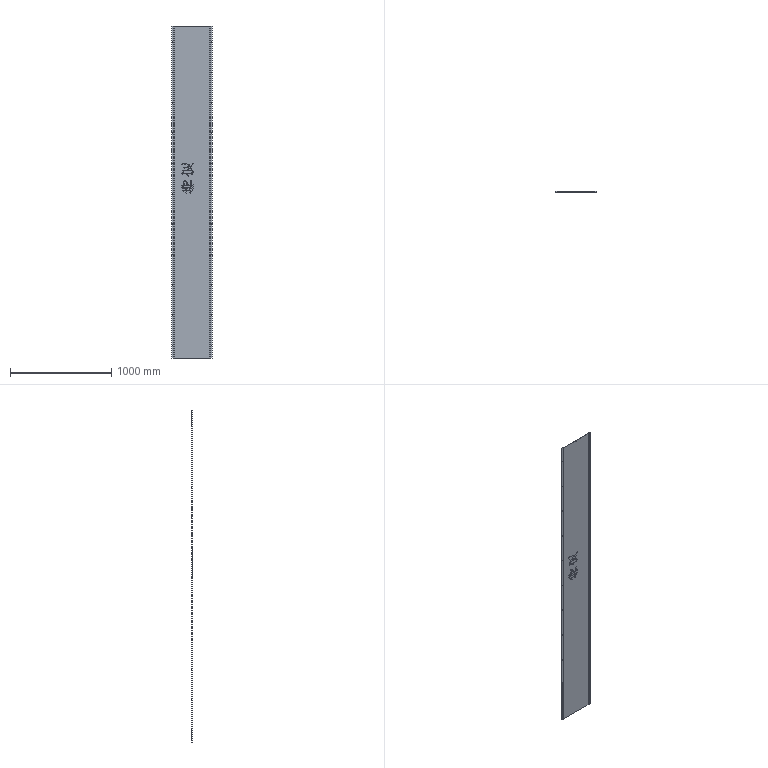Part | STEP file | TS-S87 TBD | 1 solid | 193 faces | box 402 x 4.3 x 3283 mm | volume 1592924 mm3 | plane 106 | cylinder 54 | spline 33 | commonest cylinder face diameters 5.4 x44 0.4 x4 2.8 x4 10 x2